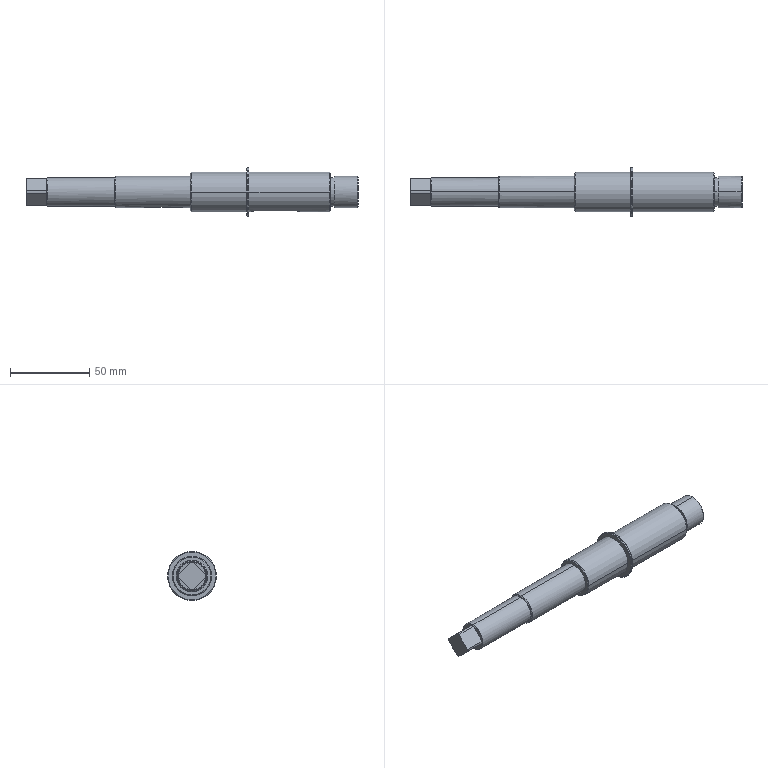Part | NX | 1 solid | 58 faces | box 210 x 31 x 31 mm | volume 75859 mm3 | cylinder 25 | plane 19 | cone 14 | commonest cylinder face diameters 17 x5 18 x4 20 x4 25 x4 6 x3 8 x3